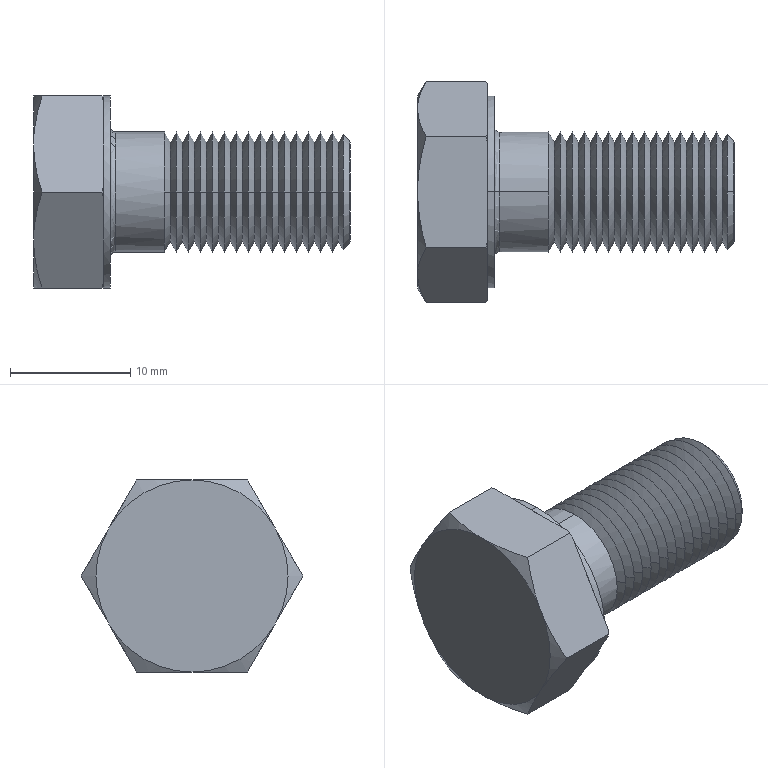Part | SolidWorks | features RevCut 4, Chamfer 1, Extrusion 1, Fillet 1, LPattern 1, Revolution 1 | 1 solid | 125 faces | box 26.4 x 18.475 x 16 mm | volume 2773 mm3 | cone 76 | cylinder 32 | plane 15 | torus 2 | commonest cylinder face diameters 10 x30 16 x2